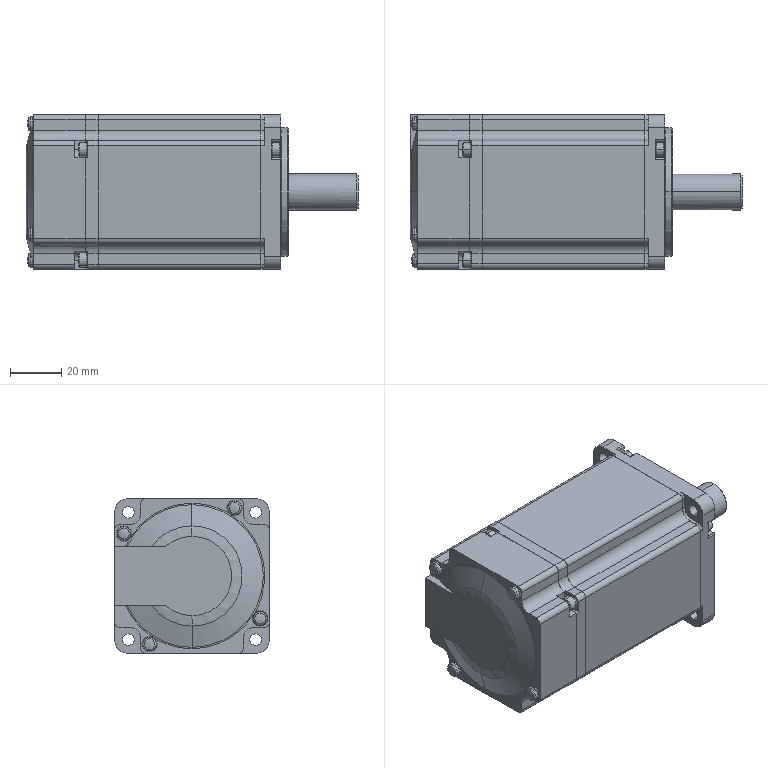Part | SolidWorks | features BaseBody 1 | 1 solid | 435 faces | box 129 x 60 x 60 mm | volume 324718 mm3 | plane 219 | cylinder 165 | cone 31 | spline 20 | commonest cylinder face diameters 4 x32 6 x24 3.92 x20 5.5 x16 8 x16 6.5 x13